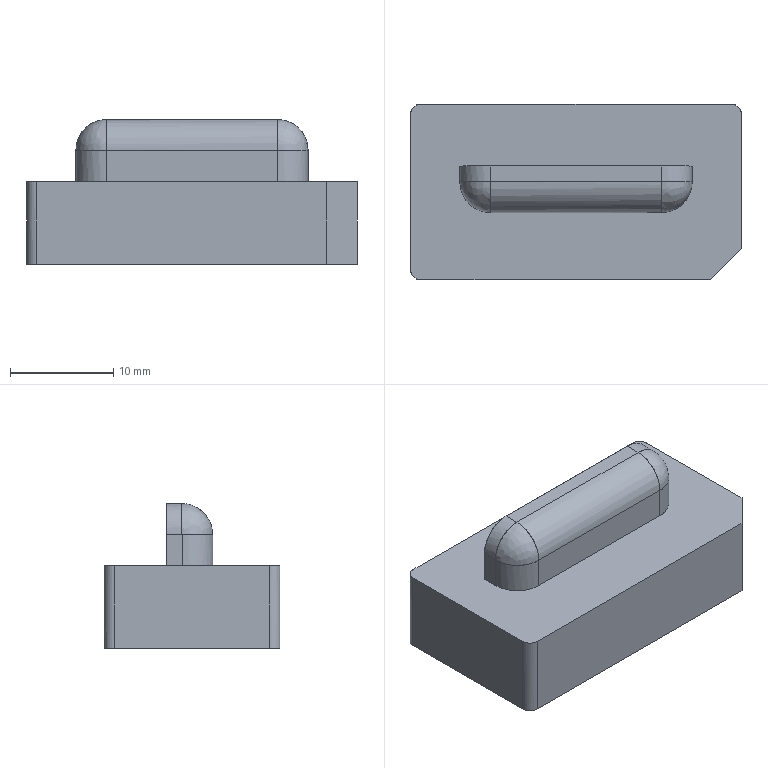NC program | PowerMill | posted with a generic post | part box 32 x 17 x 14 mm
Lines 2418 to 3447 of 64476:
N2515 M6
N2516 S18000 M03
N2517 G00 G90 X0.0 Y0.0
N2518 G43 Z9.8 H2
N2519
N2520 G05 P10000 R4
N2521 X-1.4376 Y5.4648
N2522 Z0.7927
N2523 G01 Z-0.4073 F3600.0
N2524 X-1.4475 Y5.4451 F6000.0
N2525 G03 X-1.3589 Y5.1795 I0.1771 J-0.0885
N2526 G01 X0.0 Y4.5
N2527 X9.273
N2528 X9.7611 Y4.4568
N2529 X10.2491 Y4.285
N2530 X10.4804 Y4.1484
N2531 X10.7372 Y3.9401
N2532 X10.9771 Y3.6604
N2533 X11.2333 Y3.1723
N2534 X11.3397 Y2.6843
N2535 X11.3396 Y0.7321
N2536 X11.2436 Y0.244
N2537 X11.0704 Y-0.244
N2538 X10.7372 Y-0.8496
N2539 X10.4109 Y-1.2201
N2540 X10.2491 Y-1.3547
N2541 X9.7202 Y-1.7082
N2542 X9.273 Y-1.9148
N2543 X8.7849 Y-2.0298
N2544 X8.2969 Y-2.0906
N2545 X7.8088 Y-2.076
N2546 X7.8058
N2547 X-7.8088
N2548 X-7.8118 Y-2.0761
N2549 X-8.2969 Y-2.0906
N2550 X-8.7849 Y-2.0298
N2551 X-9.273 Y-1.9148
N2552 X-9.7213 Y-1.7082
N2553 X-10.2491 Y-1.3547
N2554 X-10.4129 Y-1.2201
N2555 X-10.7372 Y-0.8496
N2556 X-11.0703 Y-0.244
N2557 X-11.2252 Y0.1688
N2558 X-11.3359 Y0.7321
N2559 X-11.3384 Y2.6843
N2560 X-11.2252 Y3.1794
N2561 X-10.9798 Y3.6604
N2562 X-10.7372 Y3.9401
N2563 X-10.4803 Y4.1484
N2564 X-10.2491 Y4.285
N2565 X-9.7611 Y4.4568
N2566 X-9.273 Y4.5
N2567 X0.0
N2568 X-1.4387 Y5.4653 Z-0.6047
N2569 X-1.4485 Y5.4456
N2570 G03 X-1.36 Y5.1799 I0.1771 J-0.0886
N2571 G01 X0.0 Y4.4999
N2572 X9.7611
N2573 X10.2491 Y4.4358
N2574 X10.7372 Y4.2379
N2575 X10.8806 Y4.1484
N2576 X11.2252 Y3.8482
N2577 X11.377 Y3.6604
N2578 X11.6317 Y3.1723
N2579 X11.7396 Y2.6843
N2580 X11.7475 Y0.7321
N2581 X11.6705 Y0.244
N2582 X11.5146 Y-0.244
N2583 X11.2879 Y-0.7321
N2584 X10.9613 Y-1.2201
N2585 X10.7372 Y-1.4639
N2586 X10.2491 Y-1.8721
N2587 X9.6545 Y-2.1962
N2588 X9.273 Y-2.3575
N2589 X8.7849 Y-2.4531
N2590 X8.2969 Y-2.501
N2591 X7.8088 Y-2.4769
N2592 X7.804
N2593 X-7.8088
N2594 X-7.8138 Y-2.4772
N2595 X-8.2969 Y-2.501
N2596 X-8.7849 Y-2.4534
N2597 X-9.273 Y-2.3575
N2598 X-9.6529 Y-2.1962
N2599 X-10.2491 Y-1.8721
N2600 X-10.7372 Y-1.4639
N2601 X-10.9574 Y-1.2201
N2602 X-11.2252 Y-0.8416
N2603 X-11.5141 Y-0.244
N2604 X-11.6705 Y0.244
N2605 X-11.7473 Y0.7321
N2606 X-11.7396 Y2.6843
N2607 X-11.6316 Y3.1723
N2608 X-11.3774 Y3.6604
N2609 X-11.2252 Y3.8482
N2610 X-10.8806 Y4.1484
N2611 X-10.7372 Y4.2379
N2612 X-10.2491 Y4.4358
N2613 X-9.7611 Y4.4999
N2614 X0.0
N2615 X-1.4387 Y5.4653 Z-0.802
N2616 X-1.4485 Y5.4456
N2617 G03 X-1.36 Y5.1799 I0.1771 J-0.0886
N2618 G01 X0.0 Y4.5
N2619 X9.7611
N2620 X10.2491 Y4.4888
N2621 X10.7372 Y4.378
N2622 X11.1849 Y4.1484
N2623 X11.6813 Y3.6604
N2624 X11.936 Y3.1723
N2625 X12.0439 Y2.6843
N2626 X12.0341 Y0.7321
N2627 X11.9695 Y0.244
N2628 X11.8413 Y-0.244
N2629 X11.6383 Y-0.7321
N2630 X11.3306 Y-1.2201
N2631 X10.9275 Y-1.7082
N2632 X10.7372 Y-1.8885
N2633 X10.2491 Y-2.2209
N2634 X9.7611 Y-2.4797
N2635 X9.1881 Y-2.6843
N2636 X8.7849 Y-2.7561
N2637 X8.2969 Y-2.7974
N2638 X7.8088 Y-2.7842
N2639 X7.8062
N2640 X-7.8088
N2641 X-7.8115 Y-2.7843
N2642 X-8.2969 Y-2.7974
N2643 X-8.7849 Y-2.7556
N2644 X-9.1897 Y-2.6843
N2645 X-9.7611 Y-2.4797
N2646 X-10.2491 Y-2.2209
N2647 X-10.7372 Y-1.8885
N2648 X-10.9281 Y-1.7082
N2649 X-11.3309 Y-1.2201
N2650 X-11.6379 Y-0.7321
N2651 X-11.8395 Y-0.244
N2652 X-11.9696 Y0.244
N2653 X-12.0349 Y0.7321
N2654 X-12.0424 Y2.6843
N2655 X-11.9359 Y3.1723
N2656 X-11.7133 Y3.6134
N2657 X-11.2252 Y4.118
N2658 X-10.7372 Y4.378
N2659 X-10.2491 Y4.4888
N2660 X-9.7611 Y4.5
N2661 X0.0
N2662 X-1.4382 Y5.465 Z-0.9993
N2663 X-1.4481 Y5.4454
N2664 G03 X-1.3595 Y5.1797 I0.1771 J-0.0886
N2665 G01 X0.0 Y4.5
N2666 X10.2491
N2667 X10.7372 Y4.448
N2668 X11.2252 Y4.264
N2669 X11.4179 Y4.1484
N2670 X11.7133 Y3.8996
N2671 X11.9143 Y3.6604
N2672 X12.1689 Y3.1723
N2673 X12.2768 Y2.6843
N2674 X12.2727 Y0.7321
N2675 X12.2127 Y0.244
N2676 X12.0961 Y-0.244
N2677 X11.8955 Y-0.7321
N2678 X11.6182 Y-1.2201
N2679 X11.2252 Y-1.7254
N2680 X10.7296 Y-2.1962
N2681 X10.2491 Y-2.5
N2682 X9.8961 Y-2.6843
N2683 X9.273 Y-2.8957
N2684 X8.7849 Y-2.9901
N2685 X8.2969 Y-3.0342
N2686 X7.8088 Y-3.0246
N2687 X7.8069
N2688 X-7.8088
N2689 X-7.8108 Y-3.0247
N2690 X-8.2969 Y-3.0342
N2691 X-8.7849 Y-2.9916
N2692 X-9.273 Y-2.8957
N2693 X-9.7611 Y-2.7419
N2694 X-10.2491 Y-2.5
N2695 X-10.7372 Y-2.1877
N2696 X-11.2425 Y-1.7082
N2697 X-11.6178 Y-1.2201
N2698 X-11.895 Y-0.7321
N2699 X-12.0959 Y-0.244
N2700 X-12.2013 Y0.1819
N2701 X-12.2725 Y0.7321
N2702 X-12.2765 Y2.6843
N2703 X-12.1688 Y3.1723
N2704 X-11.9131 Y3.6604
N2705 X-11.7133 Y3.8996
N2706 X-11.4169 Y4.1484
N2707 X-11.2252 Y4.264
N2708 X-10.7372 Y4.448
N2709 X-10.2491 Y4.5
N2710 X0.0
N2711 X-1.4387 Y5.4653 Z-1.1967
N2712 X-1.4486 Y5.4456
N2713 G03 X-1.36 Y5.18 I0.1771 J-0.0885
N2714 G01 X0.0 Y4.5
N2715 X10.2491
N2716 X10.7372 Y4.4822
N2717 X11.2252 Y4.3534
N2718 X11.7133 Y4.0692
N2719 X12.103 Y3.6604
N2720 X12.2013 Y3.5078
N2721 X12.3577 Y3.1723
N2722 X12.4655 Y2.6843
N2723 X12.47 Y0.7321
N2724 X12.4072 Y0.244
N2725 X12.2013 Y-0.4987
N2726 X11.858 Y-1.2201
N2727 X11.4981 Y-1.7082
N2728 X11.2252 Y-2.0162
N2729 X10.7372 Y-2.4193
N2730 X10.3248 Y-2.6843
N2731 X9.7611 Y-2.9562
N2732 X8.9222 Y-3.1723
N2733 X8.2969 Y-3.2286
N2734 X7.8088 Y-3.2172
N2735 X7.8065
N2736 X-7.8088
N2737 X-7.8112 Y-3.2173
N2738 X-8.2969 Y-3.2286
N2739 X-8.9255 Y-3.1723
N2740 X-9.7611 Y-2.9562
N2741 X-10.2491 Y-2.7264
N2742 X-10.7372 Y-2.4193
N2743 X-11.2252 Y-2.0162
N2744 X-11.4979 Y-1.7082
N2745 X-11.858 Y-1.2201
N2746 X-12.2013 Y-0.4987
N2747 X-12.4072 Y0.244
N2748 X-12.47 Y0.7321
N2749 X-12.4651 Y2.6843
N2750 X-12.3574 Y3.1723
N2751 X-12.2013 Y3.5078
N2752 X-12.103 Y3.6604
N2753 X-11.7133 Y4.0692
N2754 X-11.2252 Y4.3534
N2755 X-10.7372 Y4.4822
N2756 X-10.2491 Y4.5
N2757 X0.0
N2758 X-1.4388 Y5.4653 Z-1.394
N2759 X-1.4487 Y5.4456
N2760 G03 X-1.3601 Y5.18 I0.1771 J-0.0885
N2761 G01 X0.0 Y4.4999
N2762 X10.2491
N2763 X10.3288 Y4.497
N2764 X10.7372
N2765 X11.2252 Y4.4123
N2766 X11.7133 Y4.1876
N2767 X12.2013 Y3.7503
N2768 X12.2702 Y3.6604
N2769 X12.5248 Y3.1723
N2770 X12.6327 Y2.6843
N2771 X12.626 Y0.7321
N2772 X12.5712 Y0.244
N2773 X12.4639 Y-0.244
N2774 X12.283 Y-0.7321
N2775 X12.0337 Y-1.2201
N2776 X11.711 Y-1.7082
N2777 X11.2727 Y-2.1962
N2778 X10.7372 Y-2.6148
N2779 X10.2491 Y-2.9066
N2780 X9.6278 Y-3.1723
N2781 X9.273 Y-3.269
N2782 X8.7849 Y-3.3588
N2783 X8.2969 Y-3.3913
N2784 X7.8088 Y-3.3797
N2785 X-7.8088
N2786 X-8.2969 Y-3.3913
N2787 X-8.7849 Y-3.3583
N2788 X-9.273 Y-3.269
N2789 X-9.6268 Y-3.1723
N2790 X-10.2491 Y-2.9066
N2791 X-10.6378 Y-2.6843
N2792 X-11.2252 Y-2.2439
N2793 X-11.7133 Y-1.7065
N2794 X-12.0323 Y-1.2201
N2795 X-12.2013 Y-0.9107
N2796 X-12.4632 Y-0.244
N2797 X-12.5708 Y0.244
N2798 X-12.626 Y0.7321
N2799 X-12.6319 Y2.6843
N2800 X-12.5241 Y3.1723
N2801 X-12.2702 Y3.6604
N2802 X-12.2013 Y3.7503
N2803 X-11.7737 Y4.1484
N2804 X-11.2252 Y4.4123
N2805 X-10.7372 Y4.497
N2806 X-10.3288
N2807 X-10.3252 Y4.4971
N2808 X-10.2491 Y4.4999
N2809 X0.0
N2810 X-1.4388 Y5.4653 Z-1.5913
N2811 X-1.4486 Y5.4456
N2812 G03 X-1.3601 Y5.18 I0.1771 J-0.0885
N2813 G01 X0.0 Y4.4999
N2814 X10.7372
N2815 X11.2252 Y4.4477
N2816 X11.7133 Y4.2643
N2817 X11.904 Y4.1484
N2818 X12.2013 Y3.8982
N2819 X12.4005 Y3.6604
N2820 X12.6561 Y3.1723
N2821 X12.7633 Y2.6843
N2822 X12.7709 Y0.7321
N2823 X12.7132 Y0.244
N2824 X12.5966 Y-0.244
N2825 X12.4294 Y-0.7321
N2826 X12.2013 Y-1.2151
N2827 X11.7133 Y-1.9309
N2828 X11.2252 Y-2.4167
N2829 X10.8835 Y-2.6843
N2830 X10.2491 Y-3.0652
N2831 X9.9985 Y-3.1723
N2832 X9.7611 Y-3.2705
N2833 X9.273 Y-3.4034
N2834 X8.7849 Y-3.4911
N2835 X8.2969 Y-3.5291
N2836 X7.8081 Y-3.5254
N2837 X7.8074
N2838 X-7.3208
N2839 X-8.2969 Y-3.5291
N2840 X-8.7849 Y-3.4905
N2841 X-9.273 Y-3.4034
N2842 X-9.7611 Y-3.2705
N2843 X-10.2491 Y-3.0652
N2844 X-10.7372 Y-2.7863
N2845 X-11.2252 Y-2.4167
N2846 X-11.7133 Y-1.9309
N2847 X-12.2013 Y-1.2151
N2848 X-12.4293 Y-0.7321
N2849 X-12.5959 Y-0.244
N2850 X-12.6894 Y0.132
N2851 X-12.7708 Y0.7321
N2852 X-12.763 Y2.6843
N2853 X-12.6551 Y3.1723
N2854 X-12.4005 Y3.6604
N2855 X-12.2013 Y3.8982
N2856 X-11.9045 Y4.1484
N2857 X-11.7133 Y4.2643
N2858 X-11.2252 Y4.4477
N2859 X-10.7372 Y4.4999
N2860 X0.0
N2861 X-1.4388 Y5.4653 Z-1.7887
N2862 X-1.4486 Y5.4456
N2863 G03 X-1.3601 Y5.18 I0.1771 J-0.0885
N2864 G01 X0.0 Y4.4999
N2865 X10.7372
N2866 X11.2252 Y4.4704
N2867 X11.7133 Y4.3213
N2868 X12.0196 Y4.1484
N2869 X12.2013 Y4.0077
N2870 X12.5165 Y3.6604
N2871 X12.6894 Y3.3657
N2872 X12.771 Y3.1723
N2873 X12.8789 Y2.6843
N2874 X12.876 Y0.7321
N2875 X12.8217 Y0.244
N2876 X12.7225 Y-0.244
N2877 X12.5514 Y-0.7321
N2878 X12.2013 Y-1.4484
N2879 X11.7133 Y-2.1028
N2880 X11.084 Y-2.6843
N2881 X10.2978 Y-3.1723
N2882 X9.7611 Y-3.399
N2883 X9.273 Y-3.5278
N2884 X8.7849 Y-3.612
N2885 X8.2969 Y-3.6447
N2886 X7.8088 Y-3.6309
N2887 X7.8061
N2888 X-7.8088
N2889 X-7.8117 Y-3.631
N2890 X-8.2969 Y-3.6447
N2891 X-8.7849 Y-3.612
N2892 X-9.273 Y-3.5278
N2893 X-9.7611 Y-3.399
N2894 X-10.2983 Y-3.1723
N2895 X-11.0832 Y-2.6843
N2896 X-11.6269 Y-2.1962
N2897 X-12.2013 Y-1.4484
N2898 X-12.5514 Y-0.7321
N2899 X-12.6894 Y-0.3677
N2900 X-12.8213 Y0.244
N2901 X-12.8755 Y0.7321
N2902 X-12.8791 Y2.6843
N2903 X-12.771 Y3.1723
N2904 X-12.6894 Y3.3657
N2905 X-12.5154 Y3.6604
N2906 X-12.2013 Y4.0077
N2907 X-12.0199 Y4.1484
N2908 X-11.7133 Y4.3213
N2909 X-11.2252 Y4.4704
N2910 X-10.7372 Y4.4999
N2911 X0.0
N2912 X-1.4285 Y5.4602 Z-1.986
N2913 X-1.4384 Y5.4405
N2914 G03 X-1.3498 Y5.1749 I0.1771 J-0.0886
N2915 G01 X0.0 Y4.4999
N2916 X10.7372
N2917 X11.2252 Y4.4851
N2918 X11.7133 Y4.3621
N2919 X12.2013 Y4.0857
N2920 X12.6114 Y3.6604
N2921 X12.8657 Y3.1723
N2922 X12.974 Y2.6843
N2923 X12.9775 Y0.7321
N2924 X12.9213 Y0.244
N2925 X12.8122 Y-0.244
N2926 X12.6894 Y-0.6464
N2927 X12.43 Y-1.2201
N2928 X12.2013 Y-1.6248
N2929 X11.7133 Y-2.2378
N2930 X11.234 Y-2.6843
N2931 X10.7372 Y-3.0331
N2932 X10.2491 Y-3.3008
N2933 X9.7611 Y-3.4932
N2934 X9.1011 Y-3.6604
N2935 X8.2969 Y-3.7426
N2936 X7.8088 Y-3.7364
N2937 X7.8076
N2938 X-7.8088
N2939 X-7.8101
N2940 X-8.2969 Y-3.7426
N2941 X-9.101 Y-3.6604
N2942 X-9.7611 Y-3.4932
N2943 X-10.2491 Y-3.3008
N2944 X-10.7372 Y-3.0331
N2945 X-11.2252 Y-2.6911
N2946 X-11.7133 Y-2.2378
N2947 X-12.1448 Y-1.7082
N2948 X-12.4291 Y-1.2201
N2949 X-12.6583 Y-0.7321
N2950 X-12.8117 Y-0.244
N2951 X-12.9207 Y0.244
N2952 X-12.978 Y0.7321
N2953 X-12.9742 Y2.6843
N2954 X-12.8661 Y3.1723
N2955 X-12.6121 Y3.6604
N2956 X-12.2013 Y4.0857
N2957 X-11.7133 Y4.3621
N2958 X-11.2252 Y4.4851
N2959 X-10.7372 Y4.4999
N2960 X0.0
N2961 X-1.4329 Y5.4624 Z-2.1833
N2962 X-1.4428 Y5.4427
N2963 G03 X-1.3542 Y5.1771 I0.1771 J-0.0885
N2964 G01 X0.0 Y4.4999
N2965 X10.7372
N2966 X11.2252 Y4.4927
N2967 X11.7133 Y4.3892
N2968 X12.2013 Y4.1402
N2969 X12.6849 Y3.6604
N2970 X12.9396 Y3.1723
N2971 X13.0474 Y2.6843
N2972 X13.0464 Y0.7321
N2973 X12.9967 Y0.244
N2974 X12.9008 Y-0.244
N2975 X12.7368 Y-0.7321
N2976 X12.526 Y-1.2201
N2977 X12.2013 Y-1.7587
N2978 X11.8529 Y-2.1962
N2979 X11.3509 Y-2.6843
N2980 X10.7372 Y-3.1269
N2981 X10.2491 Y-3.3937
N2982 X9.4842 Y-3.6604
N2983 X8.7849 Y-3.7876
N2984 X8.2969 Y-3.8208
N2985 X7.8088 Y-3.8115
N2986 X7.807
N2987 X-7.8088
N2988 X-7.8108
N2989 X-8.2969 Y-3.8208
N2990 X-8.7849 Y-3.7874
N2991 X-9.273 Y-3.7057
N2992 X-9.7611 Y-3.5796
N2993 X-10.2491 Y-3.3937
N2994 X-10.6595 Y-3.1723
N2995 X-11.2252 Y-2.7868
N2996 X-11.7133 Y-2.3505
N2997 X-12.2013 Y-1.7587
N2998 X-12.5256 Y-1.2201
N2999 X-12.6894 Y-0.8531
N3000 X-12.9003 Y-0.244
N3001 X-12.9968 Y0.244
N3002 X-13.0471 Y0.7321
N3003 X-13.0474 Y2.6843
N3004 X-12.9403 Y3.1723
N3005 X-12.6853 Y3.6604
N3006 X-12.2013 Y4.1402
N3007 X-11.7133 Y4.3892
N3008 X-11.2252 Y4.4927
N3009 X-10.7372 Y4.4999
N3010 X0.0
N3011 X-1.4374 Y5.4646 Z-2.3807
N3012 X-1.4473 Y5.4449
N3013 G03 X-1.3587 Y5.1793 I0.1771 J-0.0885
N3014 G01 X0.0 Y4.4999
N3015 X10.7372
N3016 X10.9416 Y4.4969
N3017 X11.2252 Y4.4968
N3018 X11.7133 Y4.4093
N3019 X12.2013 Y4.1812
N3020 X12.6894 Y3.7369
N3021 X13.0011 Y3.1723
N3022 X13.1094 Y2.6843
N3023 X13.1147 Y0.7321
N3024 X13.0598 Y0.244
N3025 X12.9582 Y-0.244
N3026 X12.8057 Y-0.7321
N3027 X12.5949 Y-1.2201
N3028 X12.304 Y-1.7082
N3029 X11.9378 Y-2.1962
N3030 X11.4619 Y-2.6843
N3031 X10.7858 Y-3.1723
N3032 X10.2491 Y-3.4588
N3033 X9.7118 Y-3.6604
N3034 X9.273 Y-3.7693
N3035 X8.7849 Y-3.851
N3036 X8.2969 Y-3.8832
N3037 X7.8088 Y-3.8714
N3038 X-7.8088
N3039 X-7.8112
N3040 X-8.2969 Y-3.8832
N3041 X-8.7849 Y-3.8508
N3042 X-9.273 Y-3.7693
N3043 X-9.7124 Y-3.6604
N3044 X-10.2491 Y-3.4588
N3045 X-10.7863 Y-3.1723
N3046 X-11.4618 Y-2.6843
N3047 X-11.7133 Y-2.4428
N3048 X-12.2013 Y-1.863
N3049 X-12.5946 Y-1.2201
N3050 X-12.8065 Y-0.7321
N3051 X-12.9588 Y-0.244
N3052 X-13.0601 Y0.244
N3053 X-13.115 Y0.7321
N3054 X-13.1094 Y2.6843
N3055 X-13.0011 Y3.1723
N3056 X-12.7465 Y3.6604
N3057 X-12.2501 Y4.1484
N3058 X-11.7133 Y4.4093
N3059 X-11.2252 Y4.4968
N3060 X-10.7372 Y4.5
N3061 X-10.3541 Y4.4999
N3062 X0.0
N3063 X-1.4388 Y5.4652 Z-2.578
N3064 X-1.4487 Y5.4456
N3065 G03 X-1.3601 Y5.1799 I0.1771 J-0.0886
N3066 G01 X0.0 Y4.4998
N3067 X10.7372
N3068 X10.809 Y4.4988
N3069 X10.8105
N3070 X11.2252
N3071 X11.7133 Y4.4246
N3072 X12.3015 Y4.1484
N3073 X12.6894 Y3.7998
N3074 X12.7962 Y3.6604
N3075 X13.0496 Y3.1723
N3076 X13.1585 Y2.6843
N3077 X13.1552 Y0.7321
N3078 X13.1098 Y0.244
N3079 X13.0066 Y-0.244
N3080 X12.8629 Y-0.7321
N3081 X12.6894 Y-1.1234
N3082 X12.3669 Y-1.7082
N3083 X12.0066 Y-2.1962
N3084 X11.5356 Y-2.6843
N3085 X10.8945 Y-3.1723
N3086 X10.2491 Y-3.5156
N3087 X9.8581 Y-3.6604
N3088 X9.273 Y-3.8201
N3089 X8.7849 Y-3.9005
N3090 X8.2969 Y-3.9328
N3091 X-8.2969
N3092 X-8.7849 Y-3.9005
N3093 X-9.273 Y-3.8201
N3094 X-9.7611 Y-3.6954
N3095 X-10.2491 Y-3.5156
N3096 X-10.8946 Y-3.1723
N3097 X-11.5353 Y-2.6843
N3098 X-12.0068 Y-2.1962
N3099 X-12.3664 Y-1.7082
N3100 X-12.6431 Y-1.2201
N3101 X-12.8624 Y-0.7321
N3102 X-13.0073 Y-0.244
N3103 X-13.11 Y0.244
N3104 X-13.1552 Y0.7321
N3105 X-13.1584 Y2.6843
N3106 X-13.0523 Y3.1723
N3107 X-12.7949 Y3.6604
N3108 X-12.6894 Y3.7998
N3109 X-12.2984 Y4.1484
N3110 X-11.7133 Y4.4246
N3111 X-11.2252 Y4.4988
N3112 X-10.912
N3113 X-10.7372 Y4.4999
N3114 X-10.3541 Y4.4998
N3115 X0.0
N3116 X-1.4389 Y5.4652 Z-2.7753
N3117 X-1.4488 Y5.4456
N3118 G03 X-1.3602 Y5.1799 I0.1771 J-0.0886
N3119 G01 X0.0 Y4.4998
N3120 X10.7372
N3121 X10.7387
N3122 X11.2252
N3123 X11.7133 Y4.4326
N3124 X12.2013 Y4.2303
N3125 X12.3305 Y4.1484
N3126 X12.6894 Y3.8317
N3127 X12.827 Y3.6604
N3128 X13.0805 Y3.1723
N3129 X13.189 Y2.6843
N3130 X13.1774 Y0.5392
N3131 X13.0483 Y-0.244
N3132 X12.8944 Y-0.7321
N3133 X12.6894 Y-1.2043
N3134 X12.411 Y-1.7082
N3135 X12.0559 Y-2.1962
N3136 X11.5848 Y-2.6843
N3137 X10.9527 Y-3.1723
N3138 X10.2491 Y-3.5523
N3139 X9.9596 Y-3.6604
N3140 X9.273 Y-3.8567
N3141 X8.7849 Y-3.9371
N3142 X8.2969 Y-3.9678
N3143 X7.8088 Y-3.9582
N3144 X-7.8088
N3145 X-7.8108
N3146 X-8.2969 Y-3.9678
N3147 X-8.7849 Y-3.9371
N3148 X-9.273 Y-3.8567
N3149 X-9.7611 Y-3.7321
N3150 X-10.2491 Y-3.5523
N3151 X-10.9526 Y-3.1723
N3152 X-11.5848 Y-2.6843
N3153 X-12.0559 Y-2.1962
N3154 X-12.4117 Y-1.7082
N3155 X-12.6813 Y-1.2201
N3156 X-12.8945 Y-0.7321
N3157 X-13.0479 Y-0.244
N3158 X-13.1774 Y0.5392
N3159 X-13.1884 Y2.6843
N3160 X-13.0821 Y3.1723
N3161 X-12.8258 Y3.6604
N3162 X-12.6894 Y3.8317
N3163 X-12.3296 Y4.1484
N3164 X-12.2013 Y4.2303
N3165 X-11.7133 Y4.4326
N3166 X-11.2252 Y4.4998
N3167 X-10.7492
N3168 X-10.7372 Y4.4999
N3169 X-10.3541 Y4.4998
N3170 X0.0
N3171 X-1.4387 Y5.4652 Z-2.9727
N3172 X-1.4485 Y5.4456
N3173 G03 X-1.36 Y5.1799 I0.1771 J-0.0886
N3174 G01 X0.0 Y4.4999
N3175 X11.2252
N3176 X11.7133 Y4.4364
N3177 X12.2013 Y4.2386
N3178 X12.3454 Y4.1484
N3179 X12.6894 Y3.8489
N3180 X12.8418 Y3.6604
N3181 X13.0965 Y3.1723
N3182 X13.2043 Y2.6843
N3183 X13.2073 Y0.7321
N3184 X13.1774 Y0.3266
N3185 X13.0694 Y-0.244
N3186 X12.9136 Y-0.7321
N3187 X12.7063 Y-1.2201
N3188 X12.4382 Y-1.7082
N3189 X12.0829 Y-2.1962
N3190 X11.7133 Y-2.5868
N3191 X10.9923 Y-3.1723
N3192 X10.2491 Y-3.5756
N3193 X10.0065 Y-3.6684
N3194 X9.7611 Y-3.7537
N3195 X9.273 Y-3.8789
N3196 X8.7849 Y-3.9572
N3197 X8.2969 Y-3.9885
N3198 X7.8088 Y-3.9776
N3199 X7.8066
N3200 X-7.8088
N3201 X-7.811 Y-3.9777
N3202 X-8.2969 Y-3.9885
N3203 X-8.7849 Y-3.957
N3204 X-9.273 Y-3.8773
N3205 X-9.7611 Y-3.7537
N3206 X-10.2491 Y-3.5756
N3207 X-10.9923 Y-3.1723
N3208 X-11.616 Y-2.6843
N3209 X-12.0845 Y-2.1962
N3210 X-12.4387 Y-1.7082
N3211 X-12.6894 Y-1.2536
N3212 X-12.9138 Y-0.7321
N3213 X-13.0694 Y-0.244
N3214 X-13.1774 Y0.3266
N3215 X-13.2077 Y0.7321
N3216 X-13.2043 Y2.6843
N3217 X-13.0965 Y3.1723
N3218 X-12.8418 Y3.6604
N3219 X-12.6894 Y3.8489
N3220 X-12.3454 Y4.1484
N3221 X-12.2013 Y4.2386
N3222 X-11.7133 Y4.4364
N3223 X-11.2252 Y4.4999
N3224 X0.0
N3225 X-1.4386 Y5.4652 Z-3.17
N3226 X-1.4484 Y5.4456
N3227 G03 X-1.3598 Y5.1799 I0.1771 J-0.0886
N3228 G01 X0.0 Y4.5
N3229 X11.2252
N3230 X11.7133 Y4.4396
N3231 X12.2013 Y4.2459
N3232 X12.3582 Y4.1484
N3233 X12.6894 Y3.863
N3234 X12.8547 Y3.6604
N3235 X13.1094 Y3.1723
N3236 X13.1774 Y2.937
N3237 X13.2172 Y2.6843
N3238 X13.2257 Y1.2201
N3239 X13.2071 Y0.8515
N3240 X13.2073 Y0.7321
N3241 X13.1876 Y0.4652
N3242 X13.1774 Y0.2638
N3243 X13.0766 Y-0.244
N3244 X12.9255 Y-0.7321
N3245 X12.72 Y-1.2201
N3246 X12.4498 Y-1.7082
N3247 X12.2013 Y-2.0548
N3248 X12.0669 Y-2.2104
N3249 X11.9268 Y-2.3611
N3250 X11.7133 Y-2.5994
N3251 X11.2252 Y-3.0154
N3252 X10.9997 Y-3.1662
N3253 X10.9923 Y-3.1723
N3254 X10.9838 Y-3.1769
N3255 X10.7372 Y-3.3419
N3256 X10.2771 Y-3.5603
N3257 X10.2724 Y-3.5629
N3258 X10.2491 Y-3.5755
N3259 X10.2281 Y-3.5836
N3260 X10.0663 Y-3.6604
N3261 X9.7611 Y-3.7679
N3262 X9.273 Y-3.8941
N3263 X8.7849 Y-3.969
N3264 X8.2969 Y-3.9987
N3265 X-8.2969
N3266 X-8.7849 Y-3.9689
N3267 X-9.273 Y-3.8895
N3268 X-9.7611 Y-3.7656
N3269 X-10.2491 Y-3.5878
N3270 X-11.0092 Y-3.1723
N3271 X-11.6282 Y-2.6843
N3272 X-12.0946 Y-2.1962
N3273 X-12.4501 Y-1.7082
N3274 X-12.7185 Y-1.2201
N3275 X-12.9221 Y-0.7321
N3276 X-13.0766 Y-0.244
N3277 X-13.1744 Y0.244
N3278 X-13.2155 Y0.7321
N3279 X-13.2172 Y2.6843
N3280 X-13.1774 Y2.937
N3281 X-13.1094 Y3.1723
N3282 X-12.8546 Y3.6604
N3283 X-12.6894 Y3.863
N3284 X-12.3582 Y4.1484
N3285 X-12.2013 Y4.2459
N3286 X-11.7133 Y4.4396
N3287 X-11.2252 Y4.5
N3288 X0.0
N3289 X-1.4386 Y5.4653 Z-3.3673
N3290 X-1.4484 Y5.4456
N3291 G03 X-1.3598 Y5.1799 I0.1771 J-0.0886
N3292 G01 X0.0 Y4.5
N3293 X11.2252
N3294 X11.7133 Y4.4396
N3295 X12.2013 Y4.2459
N3296 X12.3582 Y4.1484
N3297 X12.6894 Y3.863
N3298 X12.8547 Y3.6604
N3299 X13.1094 Y3.1723
N3300 X13.1774 Y2.937
N3301 X13.2172 Y2.6843
N3302 X13.2257 Y1.2201
N3303 X13.207 Y0.8495
N3304 X13.2072 Y0.7321
N3305 X13.188 Y0.4714
N3306 X13.1774 Y0.2614
N3307 X13.0771 Y-0.244
N3308 X12.9305 Y-0.7321
N3309 X12.7209 Y-1.2201
N3310 X12.4512 Y-1.7082
N3311 X12.2013 Y-2.0575
N3312 X12.1012 Y-2.1708
N3313 X12.0828 Y-2.1962
N3314 X12.0237 Y-2.2586
N3315 X11.7133 Y-2.6101
N3316 X11.2252 Y-3.0176
N3317 X10.7372 Y-3.3442
N3318 X10.0732 Y-3.6604
N3319 X9.7611 Y-3.7704
N3320 X9.273 Y-3.8983
N3321 X8.7849 Y-3.9707
N3322 X8.2969 Y-3.9999
N3323 X-8.2969
N3324 X-8.7849 Y-3.9707
N3325 X-9.273 Y-3.8983
N3326 X-9.7611 Y-3.7704
N3327 X-10.0732 Y-3.6604
N3328 X-10.1497 Y-3.624
N3329 X-10.1585 Y-3.6208
N3330 X-10.2491 Y-3.5878
N3331 X-10.4072 Y-3.5013
N3332 X-10.7372 Y-3.3442
N3333 X-11.0159 Y-3.1723
N3334 X-11.6299 Y-2.6843
N3335 X-12.0971 Y-2.1962
N3336 X-12.4512 Y-1.7082
N3337 X-12.6894 Y-1.2835
N3338 X-12.7116 Y-1.2327
N3339 X-12.7185 Y-1.2201
N3340 X-12.7481 Y-1.149
N3341 X-12.9304 Y-0.7321
N3342 X-13.0771 Y-0.244
N3343 X-13.1748 Y0.244
N3344 X-13.2157 Y0.7321
N3345 X-13.2172 Y2.6843
N3346 X-13.1774 Y2.937
N3347 X-13.1094 Y3.1723
N3348 X-12.8546 Y3.6604
N3349 X-12.6894 Y3.863
N3350 X-12.3582 Y4.1484
N3351 X-12.2013 Y4.2459
N3352 X-11.7133 Y4.4396
N3353 X-11.2252 Y4.5
N3354 X0.0
N3355 X-1.4386 Y5.4653 Z-3.5647
N3356 X-1.4484 Y5.4456
N3357 G03 X-1.3598 Y5.1799 I0.1771 J-0.0886
N3358 G01 X0.0 Y4.5
N3359 X11.2252
N3360 X11.7133 Y4.4396
N3361 X12.2013 Y4.2459
N3362 X12.3582 Y4.1484
N3363 X12.6894 Y3.8631
N3364 X12.8547 Y3.6604
N3365 X13.1094 Y3.1723
N3366 X13.1774 Y2.937
N3367 X13.2172 Y2.6843
N3368 X13.2257 Y1.2201
N3369 X13.207 Y0.8485
N3370 X13.2072 Y0.7321
N3371 X13.1881 Y0.4737
N3372 X13.1774 Y0.2614
N3373 X13.0771 Y-0.244
N3374 X12.9305 Y-0.7321
N3375 X12.7209 Y-1.2201
N3376 X12.4512 Y-1.7082
N3377 X12.2013 Y-2.0575
N3378 X12.1009 Y-2.1713
N3379 X12.0827 Y-2.1961
N3380 X12.0248 Y-2.2574
N3381 X11.7133 Y-2.6101
N3382 X11.2252 Y-3.0176
N3383 X10.7372 Y-3.3442
N3384 X10.0732 Y-3.6604
N3385 X9.7611 Y-3.7704
N3386 X9.273 Y-3.8983
N3387 X8.7849 Y-3.9707
N3388 X8.2969 Y-3.9999
N3389 X-8.2969
N3390 X-8.7849 Y-3.9707
N3391 X-9.273 Y-3.8983
N3392 X-9.7611 Y-3.7704
N3393 X-10.0732 Y-3.6604
N3394 X-10.1502 Y-3.6237
N3395 X-10.159 Y-3.6205
N3396 X-10.2491 Y-3.5877
N3397 X-10.4063 Y-3.5018
N3398 X-10.7372 Y-3.3442
N3399 X-11.0159 Y-3.1723
N3400 X-11.63 Y-2.6843
N3401 X-12.0971 Y-2.1962
N3402 X-12.4512 Y-1.7082
N3403 X-12.6894 Y-1.2835
N3404 X-12.7118 Y-1.2322
N3405 X-12.7184 Y-1.2201
N3406 X-12.7469 Y-1.152
N3407 X-12.9304 Y-0.7321
N3408 X-13.0771 Y-0.244
N3409 X-13.1748 Y0.244
N3410 X-13.2157 Y0.7321
N3411 X-13.2172 Y2.6843
N3412 X-13.1774 Y2.937
N3413 X-13.1094 Y3.1723
N3414 X-12.8546 Y3.6604
N3415 X-12.6894 Y3.8631
N3416 X-12.3583 Y4.1484
N3417 X-12.2013 Y4.2459
N3418 X-11.7133 Y4.4396
N3419 X-11.2252 Y4.5
N3420 X0.0
N3421 X-1.4385 Y5.4653 Z-3.762
N3422 X-1.4484 Y5.4456
N3423 G03 X-1.3598 Y5.1799 I0.1771 J-0.0886
N3424 G01 X0.0 Y4.5
N3425 X11.2252
N3426 X11.7133 Y4.4396
N3427 X12.2013 Y4.2459
N3428 X12.3582 Y4.1484
N3429 X12.6894 Y3.8631
N3430 X12.8547 Y3.6604
N3431 X13.1094 Y3.1723
N3432 X13.1774 Y2.9371
N3433 X13.2172 Y2.6843
N3434 X13.2257 Y1.2201
N3435 X13.207 Y0.8474
N3436 X13.2071 Y0.7321
N3437 X13.1882 Y0.4759
N3438 X13.1774 Y0.2614
N3439 X13.0771 Y-0.244
N3440 X12.9305 Y-0.7321
N3441 X12.7209 Y-1.2201
N3442 X12.4512 Y-1.7082
N3443 X12.2013 Y-2.0575
N3444 X12.1005 Y-2.1717
N3445 X12.0827 Y-2.1961
N3446 X12.0258 Y-2.2562
N3447 X11.7133 Y-2.6101
N3448 X11.2252 Y-3.0176
N3449 X10.7372 Y-3.3442
N3450 X10.0732 Y-3.6604
N3451 X9.7611 Y-3.7704
N3452 X9.273 Y-3.8983
N3453 X8.7849 Y-3.9707
N3454 X8.2969 Y-3.9999
N3455 X-8.2969
N3456 X-8.7849 Y-3.9707
N3457 X-9.273 Y-3.8983
N3458 X-9.7611 Y-3.7704
N3459 X-10.0732 Y-3.6604
N3460 X-10.1507 Y-3.6235
N3461 X-10.1595 Y-3.6203
N3462 X-10.249 Y-3.5877
N3463 X-10.4054 Y-3.5022
N3464 X-10.7372 Y-3.3442
N3465 X-11.0159 Y-3.1723
N3466 X-11.63 Y-2.6843
N3467 X-12.0971 Y-2.1962
N3468 X-12.4513 Y-1.7082
N3469 X-12.6894 Y-1.2835
N3470 X-12.712 Y-1.2316
N3471 X-12.7184 Y-1.2201
N3472 X-12.7456 Y-1.1549
N3473 X-12.9304 Y-0.7321
N3474 X-13.0771 Y-0.244
N3475 X-13.1748 Y0.244
N3476 X-13.2157 Y0.7321
N3477 X-13.2172 Y2.6843
N3478 X-13.1774 Y2.9371
N3479 X-13.1094 Y3.1723
N3480 X-12.8546 Y3.6604
N3481 X-12.6894 Y3.8631
N3482 X-12.3583 Y4.1484
N3483 X-12.2013 Y4.2459
N3484 X-11.7133 Y4.4396
N3485 X-11.2252 Y4.5
N3486 X0.0
N3487 X-1.4385 Y5.4653 Z-3.9593
N3488 X-1.4484 Y5.4456
N3489 G03 X-1.3598 Y5.18 I0.1771 J-0.0886
N3490 G01 X0.0 Y4.5
N3491 X11.2252
N3492 X11.7133 Y4.4396
N3493 X12.2013 Y4.2459
N3494 X12.3582 Y4.1484
N3495 X12.6894 Y3.8631
N3496 X12.8547 Y3.6604
N3497 X13.1094 Y3.1723
N3498 X13.1774 Y2.9371
N3499 X13.2172 Y2.6843
N3500 X13.2257 Y1.2201
N3501 X13.2069 Y0.8464
N3502 X13.2071 Y0.7321
N3503 X13.1883 Y0.4781
N3504 X13.1774 Y0.2614
N3505 X13.0771 Y-0.244
N3506 X12.9305 Y-0.7321
N3507 X12.7209 Y-1.2201
N3508 X12.4512 Y-1.7082
N3509 X12.2013 Y-2.0575
N3510 X12.1001 Y-2.1721
N3511 X12.0827 Y-2.1961
N3512 X12.0269 Y-2.255
N3513 X11.7133 Y-2.6101
N3514 X11.2252 Y-3.0176
N3515 X10.7372 Y-3.3442
N3516 X10.0732 Y-3.6604
N3517 X9.7611 Y-3.7704
N3518 X9.273 Y-3.8983
N3519 X8.7849 Y-3.9707
N3520 X8.2969 Y-3.9999
N3521 X-8.2969
N3522 X-8.7849 Y-3.9707
N3523 X-9.273 Y-3.8983
N3524 X-9.7611 Y-3.7704
N3525 X-10.0732 Y-3.6604
N3526 X-10.1512 Y-3.6232
N3527 X-10.1601 Y-3.62
N3528 X-10.249 Y-3.5876
N3529 X-10.4045 Y-3.5026
N3530 X-10.7372 Y-3.3442
N3531 X-11.0159 Y-3.1723
N3532 X-11.63 Y-2.6843
N3533 X-12.0971 Y-2.1962
N3534 X-12.4513 Y-1.7082
N3535 X-12.6894 Y-1.2835
N3536 X-12.7123 Y-1.2311
N3537 X-12.7184 Y-1.22
N3538 X-12.7443 Y-1.1578
N3539 X-12.9304 Y-0.7321
N3540 X-13.0771 Y-0.244
N3541 X-13.1748 Y0.244
N3542 X-13.2157 Y0.7321
N3543 X-13.2172 Y2.6843
N3544 X-13.1774 Y2.9371